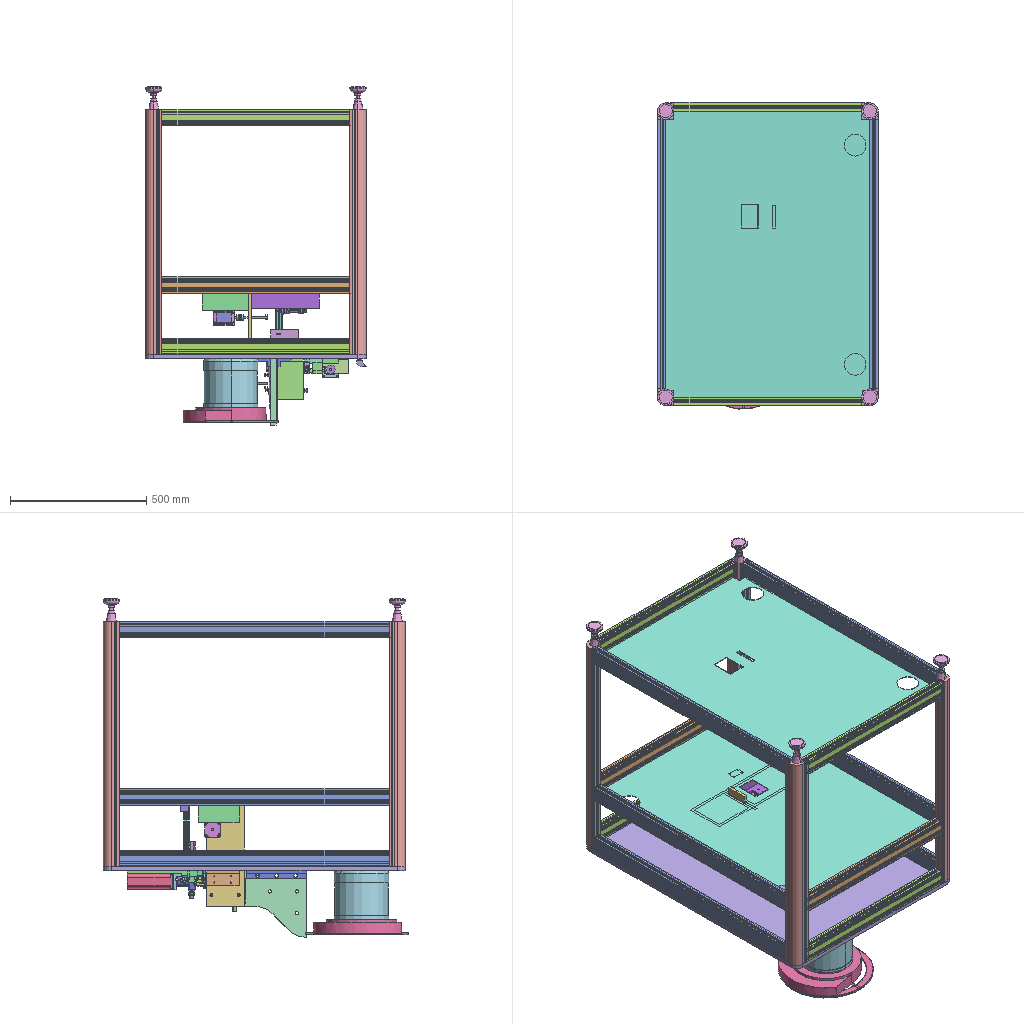Assembly | SolidWorks | 182 different items | 242 placed | box 811 x 1122 x 1244 mm
Parts list (item | name | quantity | parent item | size | volume | features):
1 | A93.step | x1 | - | - | - | -
2 | (subassembly) | x1 | - | 87.535 x 98.347 x 56.623 mm | 68756 mm3 | features Cut 3, AEMSimFeature 1, InContextFeatHolder 1
3 | (subassembly) | x1 | - | 57 x 57 x 97 mm | 225839 mm3 | -
4 | (subassembly) | x1 | - | 57 x 57 x 97 mm | 225839 mm3 | -
5 | (subassembly) | x1 | - | 282 x 25 x 285 mm | 1194987 mm3 | -
6 | (subassembly) | x3 | - | 9.63 x 17.64 x 18.86 mm | 1059 mm3 | -
7 | (subassembly) | x1 | - | 40 x 283 x 40 mm | 85274 mm3 | -
8 | (subassembly) | x1 | - | 70.171 x 19.87 x 14.369 mm | 3462 mm3 | -
9 | (subassembly) | x1 | - | 105.649 x 31.478 x 25.016 mm | 9209 mm3 | -
10 | (subassembly) | x1 | - | 105.964 x 31.504 x 25.016 mm | 9209 mm3 | -
11 | (subassembly) | x1 | - | 22.911 x 21.375 x 75.748 mm | 7166 mm3 | -
12 | (subassembly) | x1 | - | 28 x 202 x 27 mm | 86824 mm3 | -
13 | (subassembly) | x2 | - | 111 x 19.001 x 21.939 mm | 13166 mm3 | -
14 | (subassembly) | x1 | - | 5.52 x 9.1 x 11.87 mm | 178.759 mm3 | features RefPoint 2
15 | (subassembly) | x1 | - | 5.52 x 6.3 x 11.87 mm | 76.514 mm3 | features RefPoint 2
16 | (subassembly) | x3 | in 6 | 7.7 x 14.77 x 5.058 mm | 193.431 mm3 | -
17 | (subassembly) | x1 | - | 10.001 x 10 x 70 mm | 1544 mm3 | -
18 | (subassembly) | x1 | - | 10.001 x 10 x 70 mm | 1544 mm3 | -
19 | (subassembly) | x1 | - | 10.001 x 10 x 70 mm | 1544 mm3 | -
20 | (subassembly) | x1 | - | 10.001 x 10 x 70 mm | 1544 mm3 | -
21 | BODY.step | x1 | - | - | - | -
22 | - | x6 | - | 30 x 60 x 990 mm | 1191103 mm3 | features Extrusion 1
23 | - | x1 | - | 9 x 9 x 13.5 mm | 337.082 mm3 | features ICE 3, Blend 1, Extrusion 1
24 | - | x1 | - | 9 x 9 x 13.5 mm | 337.082 mm3 | features ICE 3, Blend 1, Extrusion 1
25 | - | x1 | - | 9 x 9 x 13.5 mm | 337.082 mm3 | features ICE 3, Blend 1, Extrusion 1
26 | - | x1 | - | 10 x 10 x 8.25 mm | 327.849 mm3 | features Blend 1, ICE 1
27 | - | x1 | - | 10 x 10 x 8.25 mm | 327.849 mm3 | features Blend 1, ICE 1
28 | - | x1 | - | 10 x 10 x 8.25 mm | 327.849 mm3 | features Blend 1, ICE 1
29 | - | x1 | - | 10 x 10 x 8.25 mm | 327.849 mm3 | features Blend 1, ICE 1
30 | - | x2 | - | 22 x 30 x 6 mm | 2556 mm3 | features ICE 2, Extrusion 1
31 | - | x1 | - | 4 x 4 x 70 mm | 879.646 mm3 | features Extrusion 1
32 | - | x1 | - | 4 x 4 x 70 mm | 879.646 mm3 | features Extrusion 1
33 | - | x1 | - | 22 x 7 x 22 mm | 2309 mm3 | features Revolution 1
34 | - | x1 | - | 4 x 4 x 70 mm | 879.646 mm3 | features Extrusion 1
35 | - | x1 | - | 4 x 4 x 70 mm | 879.646 mm3 | features Extrusion 1
36 | - | x1 | - | 112 x 66 x 10 mm | 42287 mm3 | features ICE 6, Extrusion 1
37 | - | x1 | - | 112 x 66 x 10 mm | 41293 mm3 | features ICE 8, Extrusion 1
38 | - | x1 | - | 53 x 47 x 12 mm | 14045 mm3 | features ICE 2, Extrusion 1
39 | - | x1 | - | 53 x 47 x 12 mm | 14009 mm3 | features ICE 4, Extrusion 1
40 | - | x3 | in 16 | 4.201 x 3.71 x 1.4 mm | 5.555 mm3 | features ICE 2, Extrusion 1, Scale 1
41 | - | x1 | - | 40 x 20 x 10 mm | 7288 mm3 | features ICE 2, Extrusion 1
42 | - | x2 | - | 36 x 30 x 8 mm | 4978 mm3 | features Extrusion 1, ICE 1
43 | - | x1 | - | 13 x 4 x 13 mm | 480.664 mm3 | features Revolution 1
44 | - | x1 | - | 22 x 7 x 22 mm | 2309 mm3 | features Revolution 1
45 | - | x1 | - | 4 x 15.2 x 4 mm | 189.539 mm3 | features Revolution 1
46 | - | x1 | - | 74 x 52 x 95 mm | 141105 mm3 | features ICE 6, Extrusion 1
47 | - | x1 | - | 5 x 19 x 58 mm | 4522 mm3 | features Extrusion 1, ICE 1
48 | - | x1 | - | 5 x 17 x 58 mm | 3929 mm3 | features Extrusion 1, ICE 1
49 | - | x1 | - | 61.5 x 23 x 10 mm | 10198 mm3 | features ICE 2, Extrusion 1
50 | - | x1 | in 7 | 15 x 15 x 8 mm | 653.451 mm3 | features Extrusion 1
51 | - | x1 | in 7 | 15 x 15 x 8 mm | 653.451 mm3 | features Extrusion 1
52 | - | x1 | in 7 | 15 x 15 x 8 mm | 653.451 mm3 | features Extrusion 1
53 | - | x1 | in 7 | 14 x 12.5 x 14 mm | 803.242 mm3 | features ICE 1, Revolution 1
54 | - | x1 | in 7 | 14 x 12.5 x 14 mm | 803.242 mm3 | features ICE 1, Revolution 1
55 | - | x1 | in 3 | 57 x 57 x 32 mm | 35611 mm3 | features BaseBody 1
56 | - | x1 | in 7 | 14 x 12.5 x 14 mm | 803.242 mm3 | features ICE 1, Revolution 1
57 | - | x1 | in 7 | 8 x 8 x 105 mm | 5097 mm3 | features ICE 2, Extrusion 1
58 | - | x1 | - | 16 x 4 x 16 mm | 603.186 mm3 | features Revolution 1
59 | - | x1 | - | 16 x 4 x 16 mm | 603.186 mm3 | features Revolution 1
60 | - | x1 | in 7 | 32 x 17 x 32 mm | 6483 mm3 | features ICE 1, Revolution 1
61 | - | x1 | - | 4 x 6 x 4 mm | 46.731 mm3 | features Revolution 1
62 | - | x1 | in 7 | 24.6 x 30 x 24.6 mm | 12751 mm3 | features Revolution 1
63 | - | x1 | - | 14 x 6 x 14 mm | 531.806 mm3 | features ICE 1, Revolution 1
64 | - | x1 | - | 14 x 6 x 14 mm | 531.806 mm3 | features ICE 1, Revolution 1
65 | - | x1 | - | 50 x 58 x 2.8 mm | 6623 mm3 | features ICE 3, Extrusion 1
66 | - | x1 | - | 112 x 67 x 16 mm | 40788 mm3 | features ICE 7, Extrusion 1
67 | - | x1 | - | 30 x 8 x 8 mm | 1687 mm3 | features ICE 2, Extrusion 1
68 | - | x2 | - | 1105 x 806 x 2 mm | 1722946 mm3 | features Cut 2, Extrusion 1
69 | - | x1 | - | 140 x 400 x 10 mm | 539172 mm3 | features Cut 1, Extrusion 1, ICE 1
70 | - | x1 | - | 50 x 55 x 121 mm | 113842 mm3 | features Cut 1, Extrusion 1, ICE 1
71 | - | x3 | - | 8 x 8 x 100 mm | 3801 mm3 | features Extrusion 1, ICE 1
72 | - | x1 | - | 23 x 42 x 35 mm | 27191 mm3 | features ICE 2, Extrusion 1
73 | - | x1 | in 7 | 26.356 x 14.7 x 26.386 mm | 3537 mm3 | features BaseBody 2
74 | - | x1 | - | 21.332 x 14.53 x 21.332 mm | 2201 mm3 | features BaseBody 2
75 | - | x1 | - | 21.332 x 14.53 x 21.332 mm | 2201 mm3 | features BaseBody 2
76 | - | x1 | - | 21.332 x 14.53 x 21.332 mm | 2201 mm3 | features BaseBody 2
77 | - | x2 | in 2 | 4 x 8 x 8 mm | 137.312 mm3 | features BaseBody 1, Scale 1
78 | - | x1 | - | 8 x 8 x 95 mm | 2950 mm3 | features Extrusion 1, ICE 1
79 | - | x1 | - | 8 x 8 x 95 mm | 2950 mm3 | features Extrusion 1, ICE 1
80 | - | x1 | - | 60 x 196.8 x 60 mm | 510939 mm3 | features BaseBody 1
81 | - | x1 | - | 26.325 x 26.325 x 14 mm | 2835 mm3 | features MBimport 1
82 | - | x1 | - | 26.325 x 26.325 x 14 mm | 2835 mm3 | features MBimport 1
83 | - | x1 | - | 26.325 x 26.325 x 14 mm | 2835 mm3 | features MBimport 1
84 | - | x1 | - | 26.325 x 26.325 x 14 mm | 2835 mm3 | features MBimport 1
85 | - | x5 | in 3 | 6 x 3 x 6 mm | 63.932 mm3 | features BaseBody 1
86 | - | x2 | in 2 | 8 x 10 x 8 mm | 253.333 mm3 | features BaseBody 1, Scale 1
87 | - | x1 | in 2 | 8 x 14 x 8 mm | 120.77 mm3 | features BaseBody 1, Scale 1
88 | - | x1 | in 2 | 26.652 x 7.62 x 6.35 mm | 402.278 mm3 | features ICE 6, Scale 2, Extrusion 1
89 | - | x3 | in 6 | 9.63 x 17.64 x 12.7 mm | 865.254 mm3 | features ICE 8, Extrusion 1
90 | - | x1 | in 2 | 26.652 x 7.62 x 6.35 mm | 402.278 mm3 | features ICE 6, Scale 2, Extrusion 1
91 | - | x1 | - | 340 x 690 x 2 mm | 469200 mm3 | features Extrusion 1
92 | - | x4 | - | 30 x 14.3 x 10 mm | 1395 mm3 | features Cut 1, Extrusion 1
93 | - | x2 | in 2 | 16 x 6 x 15.738 mm | 679.95 mm3 | features MBimport 1, RefAxis 1
94 | - | x1 | in 2 | 41.924 x 6 x 41.924 mm | 6820 mm3 | features BaseBody 1, RefAxis 1
95 | - | x1 | - | 990 x 340 x 2 mm | 673200 mm3 | features Extrusion 1
96 | - | x1 | - | 380 x 690 x 2 mm | 524400 mm3 | features Extrusion 1
97 | - | x1 | - | 35 x 42 x 20 mm | 19935 mm3 | features ICE 4, Extrusion 1
98 | - | x1 | - | 35 x 42 x 20 mm | 19935 mm3 | features ICE 4, Extrusion 1
99 | - | x1 | - | 250 x 55 x 150 mm | 687196 mm3 | features ICE 2, Cut 1, Extrusion 1
100 | - | x2 | in 14 | 3.28 x 3.28 x 3.1 mm | 13.314 mm3 | features Extrusion 1
101 | - | x1 | in 2 | 2 x 2 x 13 mm | 24.347 mm3 | features Extrusion 1, ICE 1
102 | - | x1 | in 2 | 2 x 2 x 13 mm | 24.347 mm3 | features Extrusion 1, ICE 1
103 | - | x1 | in 2 | 27 x 80 x 3 mm | 6449 mm3 | features Cut 1, Extrusion 1
104 | - | x1 | in 2 | 2.63 x 1.5 x 3.175 mm | 8.931 mm3 | features Extrusion 1, ICE 1
105 | - | x1 | in 2 | 2.632 x 1.5 x 3.175 mm | 8.936 mm3 | features Extrusion 1, ICE 1
106 | - | x1 | in 2 | 2.63 x 1.5 x 3.175 mm | 8.931 mm3 | features Extrusion 1, ICE 1
107 | - | x1 | in 2 | 2.632 x 1.5 x 3.175 mm | 8.936 mm3 | features Extrusion 1, ICE 1
108 | - | x1 | in 2 | 4.5 x 4.5 x 16.35 mm | 145.78 mm3 | features Extrusion 1, ICE 1
109 | - | x3 | in 16 | 6.79 x 10.36 x 3.938 mm | 78.166 mm3 | features ICE 21, MirrorPattern 4, Chamfer 2, MoveFace 2, Extrusion 1, Fillet 1, Scale 1
110 | - | x3 | in 16 | 2.7 x 7.8 x 2.7 mm | 7.972 mm3 | features Helix 1, RefAxis 1, Sweep 1
111 | - | x4 | in 14, 15 | 11.87 x 0.8 x 5.52 mm | 38.257 mm3 | features Extrusion 1
112 | - | x1 | - | 68.5 x 46 x 23.69 mm | 23903 mm3 | features ICE 9, Extrusion 1
113 | - | x1 | in 7 | 40 x 40 x 40 mm | 44793 mm3 | features ICE 4, Extrusion 1
114 | - | x1 | in 7 | 10 x 140 x 10 mm | 8243 mm3 | features ICE 1, Revolution 1
115 | - | x2 | - | 25 x 19 x 25 mm | 4058 mm3 | features 3DProfileFeature 1, BaseBody 1, HoleWzd 1
116 | - | x1 | in 2 | 20 x 10 x 5 mm | 819.626 mm3 | features Cut 1, MBimport 1
117 | - | x3 | - | 8.033 x 0.6 x 9.682 mm | 24.423 mm3 | features BaseBody 1
118 | - | x3 | in 16 | 7.7 x 10.5 x 4.83 mm | 101.737 mm3 | features ICE 9, Chamfer 1, Draft 1, Extrusion 1, Scale 1
119 | - | x1 | - | 8 x 74 x 8 mm | 2480 mm3 | features ICE 1, Revolution 1
120 | - | x1 | - | 17 x 5 x 17 mm | 802.52 mm3 | features Revolution 1
121 | - | x1 | - | 17 x 5 x 17 mm | 802.52 mm3 | features Revolution 1
122 | - | x1 | in 3 | 57 x 57 x 52 mm | 152457 mm3 | features BaseBody 1
123 | - | x1 | - | 1110 x 810 x 15 mm | 13214038 mm3 | features Cut 1, Extrusion 1
124 | - | x1 | in 2 | 27 x 16 x 4 mm | 1564 mm3 | features Cut 2, Extrusion 1, ICE 1
125 | - | x1 | in 2 | 27 x 16 x 4 mm | 1619 mm3 | features Cut 2, Extrusion 1
126 | - | x1 | - | 28.739 x 19.08 x 13.3 mm | 4003 mm3 | features ICE 2, BaseBody 1
127 | - | x1 | - | 17 x 5 x 17 mm | 792.467 mm3 | features Revolution 1
128 | - | x1 | - | 17 x 5 x 17 mm | 792.467 mm3 | features Revolution 1
129 | - | x1 | - | 17 x 5 x 17 mm | 792.467 mm3 | features Revolution 1
130 | - | x1 | - | 17 x 5 x 17 mm | 792.467 mm3 | features Revolution 1
131 | - | x1 | - | 68.51 x 46 x 23.69 mm | 24267 mm3 | features ICE 6, Extrusion 1
132 | - | x1 | - | 132 x 33 x 105 mm | 188680 mm3 | features ICE 12, Extrusion 1
133 | - | x1 | in 3 | 57 x 57 x 13 mm | 37451 mm3 | features BaseBody 1
134 | - | x1 | - | 374.5 x 349.5 x 236 mm | 6465739 mm3 | features ICE 7, RevCut 2, Extrusion 1, Fillet 1, Helix 1, Shell 1, Sweep 1
135 | - | x2 | - | 14 x 17.5 x 14 mm | 1918 mm3 | features BaseBody 1
136 | - | x1 | - | 25 x 6.8 x 5 mm | 756.77 mm3 | features ICE 2, Extrusion 1
137 | - | x1 | - | 25 x 6.8 x 5 mm | 756.77 mm3 | features ICE 2, Extrusion 1
138 | - | x1 | - | 25.3 x 24.8 x 15 mm | 6622 mm3 | features ICE 4, Extrusion 1
139 | - | x1 | - | 25.3 x 24.8 x 15 mm | 6622 mm3 | features ICE 4, Extrusion 1
140 | - | x1 | - | 25 x 17 x 6.5 mm | 2040 mm3 | features ICE 2, Extrusion 1
141 | - | x1 | - | 25 x 17 x 6.5 mm | 2040 mm3 | features ICE 2, Extrusion 1
142 | - | x2 | - | 15 x 33 x 15 mm | 3862 mm3 | features Revolution 1
143 | - | x1 | in 2 | 16 x 80 x 27 mm | 7781 mm3 | features ICE 2, Cut 1, Extrusion 1
144 | - | x2 | - | 30 x 60 x 690 mm | 830163 mm3 | features Extrusion 1
145 | - | x1 | in 2 | 9 x 28 x 9 mm | 895.354 mm3 | features Revolution 1
146 | - | x1 | - | 80 x 70 x 100 mm | 135093 mm3 | features Cut 3, Extrusion 1, Rib 1
147 | - | x1 | - | 80 x 70 x 100 mm | 131100 mm3 | features Cut 1, Extrusion 1
148 | - | x1 | in 2 | 31.92 x 31.92 x 54.32 mm | 39661 mm3 | features BaseBody 8, Scale 2
149 | - | x4 | - | 60 x 84 x 60 mm | 80542 mm3 | features Revolution 1
150 | - | x1 | - | 48 x 30 x 30 mm | 32140 mm3 | features ICE 3, Extrusion 1
151 | - | x1 | - | 48 x 23 x 30 mm | 22609 mm3 | features ICE 4, Extrusion 1
152 | - | x1 | - | 30 x 60 x 60 mm | 45776 mm3 | features ICE 4, Extrusion 1
153 | - | x1 | - | 480 x 60 x 16 mm | 311459 mm3 | features ICE 4, Extrusion 1
154 | - | x1 | - | 170 x 60.52 x 150 mm | 558120 mm3 | features Extrusion 1, ICE 1
155 | - | x4 | - | 30 x 60 x 690 mm | 830163 mm3 | features Extrusion 1
156 | - | x1 | in 2 | - | - | features MBimport 1
157 | - | x1 | in 2 | 12 x 12 x 3.5 mm | 150.581 mm3 | features BaseBody 4
158 | - | x3 | - | 11 x 11 x 5 mm | 259.376 mm3 | features BaseBody 4
159 | - | x1 | - | 20 x 20 x 26 mm | 5734 mm3 | features BaseBody 5
160 | - | x1 | - | 10.3 x 10.3 x 4 mm | 223.909 mm3 | features Extrusion 1, ICE 1
161 | - | x1 | - | 10.3 x 10.3 x 4 mm | 223.909 mm3 | features Extrusion 1, ICE 1
162 | - | x1 | - | 10.3 x 10.3 x 4 mm | 223.909 mm3 | features Extrusion 1, ICE 1
163 | - | x1 | - | 10.3 x 10.3 x 4 mm | 223.909 mm3 | features Extrusion 1, ICE 1
164 | - | x1 | - | 10.3 x 10.3 x 4 mm | 223.909 mm3 | features Extrusion 1, ICE 1
165 | - | x1 | - | 10.3 x 10.3 x 4 mm | 223.909 mm3 | features Extrusion 1, ICE 1
166 | - | x4 | - | 60 x 60 x 900 mm | 1580758 mm3 | features Extrusion 1
167 | - | x1 | - | 10.3 x 10.3 x 4 mm | 223.909 mm3 | features Extrusion 1, ICE 1
168 | - | x1 | - | 10.3 x 10.3 x 4 mm | 223.909 mm3 | features Extrusion 1, ICE 1
169 | - | x1 | - | 21.332 x 14.53 x 21.332 mm | 2489 mm3 | features BaseBody 2
170 | - | x1 | in 5 | 270 x 20 x 285 mm | 953710 mm3 | features Cut 3, ICE 3, Extrusion 1
171 | - | x1 | in 5 | 282 x 273 x 20 mm | 241277 mm3 | features ICE 3, Cut 2, Extrusion 1
172 | - | x1 | - | 32 x 149 x 100 mm | 140800 mm3 | features Extrusion 1
173 | - | x2 | - | 50 x 28 x 220 mm | 127251 mm3 | features Cut 4, Extrusion 1
174 | - | x2 | - | 3.85 x 51 x 80 mm | 15495 mm3 | features Cut 1, Extrusion 1
175 | - | x2 | - | 6 x 3 x 7 mm | 74.604 mm3 | features Fillet 8, ICE 3, Extrusion 1
176 | - | x1 | - | 9 x 9 x 13.5 mm | 337.082 mm3 | features ICE 3, Blend 1, Extrusion 1
177 | - | x2 | in 14 | 2.3 x 2.3 x 9.1 mm | 37.808 mm3 | features Extrusion 1
178 | HMY1B_GT1063.step | x1 | - | - | - | -
179 | HMY1B_HK1063.step | x1 | - | - | - | -
180 | SHAFT.step | x1 | - | - | - | -
181 | Partner Pneumatic_HMY1B10G-100-A93S.step (subassembly) | x1 | - | - | - | -
182 | Nuoruilang_12002-010025.step (subassembly) | x1 | - | - | - | -
Mates (type | each side: item.copy, entity, surface, feature):
In the top assembly
Coincident | 166.1 face plane Boss-Extrude 1 | 22.1 face plane Boss-Extrude 1 | 3 times
Coincident | 22.1 face plane Boss-Extrude 1 | 166.2 face plane Boss-Extrude 1 | 3 times
Coincident | 166.1 face plane Boss-Extrude 1 | 155.1 face plane Boss-Extrude 1 | 3 times
Coincident | 155.1 face plane Boss-Extrude 1 | 166.3 face plane Boss-Extrude 1 | 3 times
Coincident | 166.2 face plane Boss-Extrude 1 | 155.2 face plane Boss-Extrude 1 | 3 times
Coincident | 155.2 face plane Boss-Extrude 1 | 166.4 face plane Boss-Extrude 1 | 3 times
Coincident | 166.4 face plane Boss-Extrude 1 | 22.2 face plane Boss-Extrude 1 | 3 times
Coincident | 166.2 face plane Boss-Extrude 1 | 22.3 face plane Boss-Extrude 1 | 3 times
Coincident | 166.3 face plane Boss-Extrude 1 | 22.4 face plane Boss-Extrude 1 | 3 times
Coincident | 166.3 face plane Boss-Extrude 1 | 155.3 face plane Boss-Extrude 1 | 3 times
Coincident | 166.4 face plane Boss-Extrude 1 | 155.4 face plane Boss-Extrude 1 | 3 times
Coincident | 166.2 face plane Boss-Extrude 1 | 149.1 face plane Revolve 1
Concentric | 166.2 edge | 149.1 edge
Coincident | 166.1 face plane Boss-Extrude 1 | 149.2 face plane Revolve 1
Concentric | 166.1 edge | 149.2 edge
Coincident | 166.3 face plane Boss-Extrude 1 | 149.3 face plane Revolve 1
Concentric | 166.3 edge | 149.3 edge
Coincident | 166.4 face plane Boss-Extrude 1 | 149.4 face plane Revolve 1
Concentric | 166.4 edge | 149.4 edge
Coincident | 155.1 face plane Boss-Extrude 1 | 68.1 face plane Boss-Extrude 1
Coincident | 22.1 edge | 68.1 edge
Coincident | 155.2 edge | 68.1 edge
Coincident | 166.4 face plane Boss-Extrude 1 | 144.1 face plane Boss-Extrude 1 | 2 times
Coincident | 166.1 face plane Boss-Extrude 1 | 144.2 face plane Boss-Extrude 1 | 2 times
Coincident | 166.3 face plane Boss-Extrude 1 | 22.5 face plane Boss-Extrude 1 | 2 times
Coincident | 166.2 face plane Boss-Extrude 1 | 22.6 face plane Boss-Extrude 1 | 2 times
Coincident | 166.2 face plane Boss-Extrude 1 | 68.2 face plane Boss-Extrude 1 | 2 times
Coincident | 166.3 face plane Boss-Extrude 1 | 144.2 face plane Boss-Extrude 1 | 2 times
Coincident | 144.2 face plane Boss-Extrude 1 | 68.2 face plane Boss-Extrude 1
Coincident | 69.1 face plane Boss-Extrude 1 | 99.1 face plane Boss-Extrude 1
Coincident | 68.2 face plane Boss-Extrude 1 | 99.1 face plane Boss-Extrude 1
Coincident | 69.1 face plane Boss-Extrude 1 | 71.1 face plane Cut-Extrude 1
DistanceDim | 92.1 face plane Boss-Extrude 1 | 174.1 face plane Boss-Extrude 1
DistanceDim | 174.1 face plane Boss-Extrude 1 | 99.1 face plane Boss-Extrude 1
DistanceDim | 99.1 face plane Boss-Extrude 1 | 69.1 face plane Boss-Extrude 1
Coincident | 92.1 face plane Boss-Extrude 1 | 174.1 face plane Boss-Extrude 1
Coincident | 174.1 face plane Boss-Extrude 1 | 99.1 face plane Boss-Extrude 1
Concentric | 71.1 face cylinder Cut-Extrude 1 | 55.1 face cylinder Import 1
Concentric | 55.1 face cylinder Import 1 | 159.1 face cylinder Import 3
DistanceDim | 55.1 face plane Import 1 | 159.1 face plane Import 3
DistanceDim | 71.1 face plane Boss-Extrude 1 | 159.1 face plane Import 3
Coincident | 68.2 face plane Boss-Extrude 1 | 154.1 face plane Boss-Extrude 1
Coincident | 99.1 face plane Boss-Extrude 1 | 154.1 face plane Boss-Extrude 1
Parallel | 122.1 face plane Import 1 | 154.1 face plane Boss-Extrude 1
Coincident | 69.1 face plane Boss-Extrude 1 | 154.1 face plane Boss-Extrude 1
Concentric | 71.1 face cylinder Boss-Extrude 1 | 158.1 face cylinder Import 4
Coincident | 69.1 face plane Boss-Extrude 1 | 71.2 face plane Cut-Extrude 1
Coincident | 69.1 face plane Boss-Extrude 1 | 71.3 face plane Cut-Extrude 1
Concentric | 71.3 face cylinder Cut-Extrude 1 | 158.2 face cylinder Import 4
Concentric | 71.2 face cylinder Cut-Extrude 1 | 158.3 face cylinder Import 4
Coincident | 69.1 face plane Boss-Extrude 1 | 117.1 face plane Import 1
Coincident | 69.1 face plane Boss-Extrude 1 | 117.2 face plane Import 1
Coincident | 69.1 face plane Boss-Extrude 1 | 70.1 face plane Boss-Extrude 1 | 2 times
Coincident | 69.1 face plane Boss-Extrude 1 | 117.3 face plane Import 1
Concentric | 175.1 face cylinder Boss-Extrude 2 | 109.1 face cylinder Boss-Extrude 1
DistanceDim | 175.1 face plane Boss-Extrude 1 | 109.1 face plane Cut-Extrude 11
Coincident | 123.1 face plane Boss-Extrude 1 | 134.1 face plane Extrude 1
Coincident | 123.1 face plane Boss-Extrude 1 | 170.1 face plane Boss-Extrude 1
Coincident | 123.1 face plane Boss-Extrude 1 | 173.1 face plane Boss-Extrude 1
Coincident | 123.1 face plane Boss-Extrude 1 | 173.2 face plane Boss-Extrude 1
Coincident | 123.1 face plane Boss-Extrude 1 | 41.1 face plane Boss-Extrude 1
DistanceDim | 41.1 face plane Boss-Extrude 1 | 123.1 face plane Boss-Extrude 1
Coincident | 123.1 face plane Boss-Extrude 1 | 172.1 face plane Boss-Extrude 1
Coincident | 123.1 face plane Boss-Extrude 1 | 153.1 face plane Boss-Extrude 1
DistanceDim | 153.1 face plane Cut-Extrude 1 | 80.1 face plane Import 1
Coincident | 153.1 face plane Cut-Extrude 1 | 80.1 face plane Import 1
Coincident | 153.1 face plane Boss-Extrude 1 | 80.1 face plane Import 1
Coincident | 153.1 face plane Cut-Extrude 1 | 152.1 face plane Boss-Extrude 1
Coincident | 153.1 face plane Cut-Extrude 2 | 39.1 face plane Boss-Extrude 1 | 2 times
Concentric | 153.1 face cylinder Cut-Extrude 3 | 39.1 face cylinder Cut-Extrude 1
Coincident | 153.1 face plane Cut-Extrude 2 | 38.1 face plane Boss-Extrude 1
Concentric | 153.1 face cylinder Cut-Extrude 3 | 38.1 face cylinder Cut-Extrude 2 | 2 times
Concentric | 80.1 face cylinder Import 1 | 152.1 face cylinder Cut-Extrude 1
Coincident | 80.1 face plane Import 1 | 152.1 face plane Boss-Extrude 1
Concentric | 39.1 face cylinder Boss-Extrude 1 | 44.1 face cylinder Revolve 1
Concentric | 38.1 face cylinder Boss-Extrude 1 | 33.1 face cylinder Revolve 1
DistanceDim | 33.1 face plane Revolve 1 | 38.1 face plane Boss-Extrude 1
Coincident | 171.1 face plane Boss-Extrude 3 | 173.1 face plane Boss-Extrude 1
Coincident | 170.1 face plane Boss-Extrude 1 | 173.2 face plane Boss-Extrude 1
Coincident | 171.1 face plane Boss-Extrude 3 | 172.1 face plane Boss-Extrude 1
Coincident | 46.1 face plane Boss-Extrude 1 | 65.1 face plane Boss-Extrude 1
Concentric | 46.1 face cylinder Cut-Extrude 5 | 65.1 face cylinder Cut-Extrude 1
Concentric | 46.1 edge | 65.1 face cylinder Cut-Extrude 1
Coincident | 46.1 face plane Boss-Extrude 1 | 49.1 face plane Boss-Extrude 1
DistanceDim | 49.1 face plane Boss-Extrude 1 | 46.1 face plane Boss-Extrude 1
Concentric | 46.1 face cylinder Cut-Extrude 6 | 59.1 face cylinder Revolve 1
Coincident | 46.1 face plane Boss-Extrude 1 | 59.1 face plane Revolve 1
Concentric | 46.1 face cylinder Cut-Extrude 6 | 58.1 face cylinder Revolve 1
Coincident | 46.1 face plane Boss-Extrude 1 | 58.1 face plane Revolve 1
Concentric | 46.1 face cylinder Cut-Extrude 6 | 64.1 face cylinder Revolve 1
Coincident | 65.1 face plane Boss-Extrude 1 | 67.1 face plane Boss-Extrude 1
Concentric | 65.1 face cylinder Cut-Extrude 1 | 67.1 face cylinder Cut-Extrude 1 | 2 times
Coincident | 65.1 face plane Boss-Extrude 1 | 47.1 face plane Boss-Extrude 1
Concentric | 65.1 face cylinder Cut-Extrude 1 | 47.1 face cylinder Cut-Extrude 1 | 2 times
Coincident | 65.1 face plane Boss-Extrude 1 | 48.1 face plane Boss-Extrude 1
Concentric | 65.1 face cylinder Cut-Extrude 1 | 48.1 face cylinder Cut-Extrude 1 | 2 times
Concentric | 49.1 face cylinder Cut-Extrude 1 | 61.1 face cylinder Revolve 1
Coincident | 49.1 face plane Boss-Extrude 1 | 61.1 face plane Revolve 1
DistanceDim | 42.1 face plane Boss-Extrude 1 | 49.1 face plane Boss-Extrude 1
Coincident | 59.1 face plane Revolve 1 | 63.1 face plane Revolve 1
Coincident | 58.1 face plane Revolve 1 | 64.1 face plane Revolve 1
Coincident | 41.1 face plane Boss-Extrude 1 | 42.1 face plane Boss-Extrude 1
Concentric | 41.1 face cylinder Cut-Extrude 2 | 42.1 face cylinder Cut-Extrude 1 | 2 times
Coincident | 41.1 face plane Boss-Extrude 1 | 42.2 face plane Boss-Extrude 1
Concentric | 41.1 face cylinder Cut-Extrude 1 | 42.2 face cylinder Cut-Extrude 1 | 2 times
Parallel | 172.1 face plane Boss-Extrude 1 | 92.2 face plane Boss-Extrude 1
Parallel | 172.1 face plane Boss-Extrude 1 | 92.3 face plane Boss-Extrude 1
Coincident | 172.1 face plane Boss-Extrude 1 | 174.2 face plane Boss-Extrude 1 | 2 times
Coincident | 166.3 face plane Boss-Extrude 1 | 123.1 face plane Boss-Extrude 1
Coincident | 22.4 face plane Boss-Extrude 1 | 123.1 face plane Boss-Extrude 1
Coincident | 123.1 face plane Cut-Extrude 1 | 69.1 face plane Boss-Extrude 1
DistanceDim | 69.1 face plane Boss-Extrude 1 | 123.1 face plane Cut-Extrude 1
Coincident | 123.1 face plane Boss-Extrude 1 | 70.1 face plane Boss-Extrude 1
Parallel | 171.1 face plane Cut-Extrude 1 | 175.2 face plane Boss-Extrude 4
Coincident | 171.1 face plane Cut-Extrude 1 | 175.2 face plane Boss-Extrude 4
Concentric | 80.1 face cylinder Import 1 | 113.1 face cylinder Cut-Extrude 2
DistanceDim | 113.1 face plane Boss-Extrude 1 | 152.1 face plane Boss-Extrude 1
Concentric | 44.1 face cylinder Revolve 1 | 114.1 face cylinder Revolve 1
Coincident | 44.1 face plane Revolve 1 | 114.1 face plane Revolve 1
Concentric | 57.1 face cylinder Boss-Extrude 1 | 63.1 face cylinder Revolve 1
Concentric | 49.1 face cylinder Boss-Extrude 1 | 45.1 face cylinder Revolve 1
Coincident | 49.1 face plane Boss-Extrude 1 | 45.1 face plane Revolve 1
DistanceDim | assembly face | 123.1 face plane Boss-Extrude 1
DistanceDim | 153.1 face plane Boss-Extrude 1 | assembly face
Concentric | 45.1 face cylinder Revolve 1 | assembly face
Coincident | 49.1 face plane Cut-Extrude 2 | assembly face
Coincident | 22.5 face plane Boss-Extrude 1 | 68.2 face plane Boss-Extrude 1
Coincident | 144.1 face plane Boss-Extrude 1 | 68.2 face plane Boss-Extrude 1
Coincident | 22.6 face plane Boss-Extrude 1 | 68.2 face plane Boss-Extrude 1
Concentric | 69.1 face cylinder Cut-Extrude 2 | 158.3 face cylinder Import 3
Concentric | 71.2 face cylinder Cut-Extrude 1 | 117.2 face cylinder Import 1
Concentric | 71.3 face cylinder Cut-Extrude 1 | 117.1 face cylinder Import 1
In subassembly 7
Concentric | 114.2 face cylinder Revolve 1 | 73.1 face cylinder Yuelongda FA_G3HHB-1.0-2525-P10.step-1/ Inner.step-1-solid1
Concentric | 114.2 face cylinder Revolve 1 | 62.1 face cylinder Revolve 1
Concentric | 114.2 face cylinder Revolve 1 | 57.2 face cylinder Boss-Extrude 1
DistanceDim | 57.2 face plane Boss-Extrude 1 | 114.2 face plane Revolve 1
Concentric | 57.2 face cylinder Boss-Extrude 1 | 60.1 face cylinder Revolve 1
Coincident | 57.2 face plane Boss-Extrude 1 | 60.1 face plane Revolve 1
Concentric | 57.2 face cylinder Boss-Extrude 1 | 56.1 face cylinder Revolve 1
Concentric | 57.2 face cylinder Boss-Extrude 1 | 53.1 face cylinder Revolve 1
Concentric | 57.2 face cylinder Boss-Extrude 1 | 54.1 face cylinder Revolve 1
Concentric | 52.1 face cylinder Boss-Extrude 1 | 56.1 face cylinder Revolve 1
Coincident | 52.1 face plane Boss-Extrude 1 | 56.1 face plane Revolve 1
Concentric | 50.1 face cylinder Boss-Extrude 1 | 53.1 face cylinder Revolve 1
Coincident | 50.1 face plane Boss-Extrude 1 | 53.1 face plane Revolve 1
Concentric | 51.1 face cylinder Boss-Extrude 1 | 54.1 face cylinder Revolve 1
Coincident | 51.1 face plane Boss-Extrude 1 | 54.1 face plane Revolve 1
In subassembly 5
Coincident | 170.2 face plane Boss-Extrude 1 | 171.2 face plane Boss-Extrude 3 | 3 times
Coincident | 171.2 face plane Boss-Extrude 3 | 5.1 face
DistanceDim | 5.1 face | 170.2 face plane Boss-Extrude 1
In subassembly 15
Concentric | 111.1 face cylinder Boss-Extrude 1 | 111.2 face cylinder Boss-Extrude 1 | 2 times
DistanceDim | 111.2 face plane Boss-Extrude 1 | 111.1 face plane Boss-Extrude 1
Coincident | 111.2 axis | 15.1 plane | 2 times
DistanceDim | 111.1 axis | 15.1 plane
DistanceDim | 15.1 plane | 111.2 face plane Boss-Extrude 1
In subassembly 2
Coincident | 93.1 axis | 2.1 plane
DistanceDim | 93.1 axis | 116.1 face plane National Standard GB_GBT1356-2001_1 20 5 10_Rack.step<1>
Coincident | 93.2 axis | 2.1 plane
Concentric | 93.1 face cylinder Shanglong Automation_GEAST1.0-14-B6-H7.step<1> | 156.1 face cylinder Panqi Automation_602ZZ.step<1>
Coincident | 94.1 axis | 2.1 plane
DistanceDim | 94.1 axis | 93.1 axis
DistanceDim | 94.1 axis | 93.2 axis
Concentric | 94.1 face cylinder Import 1 | 157.1 face cylinder Import 3
Coincident | 103.1 face plane Boss-Extrude 2 | 116.1 face plane National Standard GB_GBT1356-2001_1 20 5 10_Rack.step<1>
Coincident | 103.1 face plane Boss-Extrude 2 | 93.1 face plane Shanglong Automation_GEAST1.0-14-B6-H7.step<1>
Coincident | 103.1 face plane Boss-Extrude 2 | 94.1 face plane Import 1
Coincident | 103.1 face plane Boss-Extrude 2 | 93.2 face plane Shanglong Automation_GEAST1.0-14-B6-H7.step<1>
Concentric | 143.1 face cylinder Cut-Extrude 4 | 145.1 face cylinder Revolve 19
Coincident | 143.1 face plane Boss-Extrude 1 | 145.1 face plane Revolve 19
Concentric | 103.1 face cylinder Cut-Extrude 5 | 145.1 face cylinder Revolve 19
Coincident | 103.1 face plane Boss-Extrude 2 | 143.1 face plane Boss-Extrude 1 | 2 times
LimitDistanceDim | 116.1 face plane National Standard GB_GBT1356-2001_1 20 5 10_Rack.step<1> | 143.1 face plane Boss-Extrude 1
Concentric | 87.1 face cylinder Import 1 | 77.1 face cylinder Import 1
Coincident | 87.1 face plane Import 1 | 77.1 face plane Import 1
Concentric | 87.1 face cylinder Import 1 | 77.2 face cylinder Import 1
Coincident | 87.1 face plane Import 1 | 77.2 face plane Import 1
Concentric | 77.1 face cylinder Import 1 | 86.1 face cylinder Import 1
Coincident | 77.1 face plane Import 1 | 86.1 face plane Import 1
Concentric | 77.2 face cylinder Import 1 | 86.2 face cylinder Import 1
Coincident | 77.2 face plane Import 1 | 86.2 face plane Import 1
Concentric | 86.1 face cylinder Import 1 | 145.1 face cylinder Revolve 19
DistanceDim | 86.1 face plane Import 1 | 145.1 face plane Revolve 19
Coincident | 88.1 face plane Cut-Extrude1 | 90.1 face plane Cut-Extrude1
Coincident | 88.1 face plane Boss-Extrude1 | 124.1 face plane Boss-Extrude 1
Concentric | 88.1 face cylinder Boss-Extrude1 | 90.1 face cylinder Boss-Extrude1
Concentric | 88.1 face cylinder Boss-Extrude1 | 108.1 face cylinder Boss-Extrude 1
Concentric | 88.1 face cylinder Cut-Extrude 2 | 101.1 face cylinder Boss-Extrude 1
Coincident | 88.1 face plane Cut-Extrude 4 | 106.1 face plane Boss-Extrude 1 | 2 times
Coincident | 88.1 edge | 106.1 edge
Coincident | 88.1 face plane Cut-Extrude 5 | 107.1 face plane Boss-Extrude 1
Coincident | 88.1 edge | 107.1 edge
Coincident | 88.1 face plane Boss-Extrude1 | 107.1 face plane Boss-Extrude 1
Concentric | 90.1 face cylinder Cut-Extrude 2 | 102.1 face cylinder Boss-Extrude 1
Coincident | 90.1 face plane Cut-Extrude 4 | 104.1 face plane Boss-Extrude 1 | 2 times
Coincident | 90.1 edge | 104.1 edge
Coincident | 90.1 face plane Cut-Extrude 5 | 105.1 face plane Boss-Extrude 1 | 2 times
Coincident | 90.1 edge | 105.1 edge
Coincident | 90.1 face plane Boss-Extrude1 | 125.1 face plane Boss-Extrude 1
Slot | 101.1 face cylinder Boss-Extrude 1 | 125.1 face plane Cut-Extrude 3
Slot | 102.1 face cylinder Boss-Extrude 1 | 125.1 face plane Cut-Extrude 3
Coincident | 124.1 face plane Boss-Extrude 1 | 125.1 face plane Boss-Extrude 1 | 2 times
Coincident | 103.1 face plane Boss-Extrude 2 | 125.1 face plane Boss-Extrude 1 | 3 times
Coincident | 125.1 face plane Boss-Extrude 1 | 143.1 face plane Boss-Extrude 1
Coincident | 125.1 face plane Boss-Extrude 1 | 116.1 face plane National Standard GB_GBT1356-2001_1 20 5 10_Rack.step<1>
Coincident | 108.1 face plane Boss-Extrude 1 | 116.1 face plane Cut-Extrude 1
Concentric | 108.1 face cylinder Boss-Extrude 1 | 116.1 face cylinder Cut-Extrude 1
Parallel | 103.1 face plane Boss-Extrude 2 | 86.2 face plane Import 1
Concentric | 86.2 face cylinder Import 1 | 148.1 face cylinder
Parallel | 103.1 face plane Boss-Extrude 2 | 148.1 face plane
DistanceDim | 148.1 face plane | 86.2 face plane Import 1
In subassembly 14
Concentric | 177.1 face cylinder Boss-Extrude 1 | 111.2 face cylinder Boss-Extrude 1
Concentric | 177.1 face cylinder Boss-Extrude 1 | 100.1 face cylinder Boss-Extrude 1
Coincident | 111.2 face plane Boss-Extrude 1 | 100.1 face plane Boss-Extrude 1
Concentric | 177.1 face cylinder Boss-Extrude 1 | 111.3 face cylinder Boss-Extrude 1
Coincident | 100.1 face plane Boss-Extrude 1 | 111.3 face plane Boss-Extrude 1
Concentric | 111.2 face cylinder Boss-Extrude 1 | 177.2 face cylinder Boss-Extrude 1
Concentric | 177.2 face cylinder Boss-Extrude 1 | 100.2 face cylinder Boss-Extrude 1
Coincident | 111.2 face plane Boss-Extrude 1 | 100.2 face plane Boss-Extrude 1
Concentric | 111.3 face cylinder Boss-Extrude 1 | 177.2 face cylinder Boss-Extrude 1
DistanceDim | 111.2 face plane Boss-Extrude 1 | 177.1 face plane Boss-Extrude 1
DistanceDim | 111.2 face plane Boss-Extrude 1 | 177.2 face plane Boss-Extrude 1
Coincident | 177.2 axis | 14.1 plane
Coincident | 177.1 axis | 14.1 plane
DistanceDim | 14.1 plane | 177.2 axis
DistanceDim | 111.2 face plane Boss-Extrude 1 | 14.1 plane
In subassembly 6
Coincident | 118.1 face plane Boss-Extrude 1 | 89.1 face plane Boss-Extrude 3
DistanceDim | 118.1 face plane Boss-Extrude 1 | 89.1 face plane Boss-Extrude 3
DistanceDim | 118.1 face plane Boss-Extrude 1 | 89.1 face plane Boss-Extrude 2
In subassembly 16
Concentric | 118.2 face cone Boss-Extrude 3 | 110.1 axis
Coincident | 118.2 face plane Cut-Extrude 3 | 110.1 plane
Coincident | 118.2 plane | 109.2 plane
Coincident | 118.2 face plane Cut-Extrude 1 | 109.2 face plane Boss-Extrude 1
LimitDistanceDim | 109.2 face plane Boss-Extrude 5 | 118.2 face plane Cut-Extrude 4
Concentric | 40.1 face cylinder Boss-Extrude 1 | 109.2 face cylinder Cut-Extrude 9
Coincident | 40.1 face plane Boss-Extrude 1 | 109.2 face plane Cut-Extrude 2